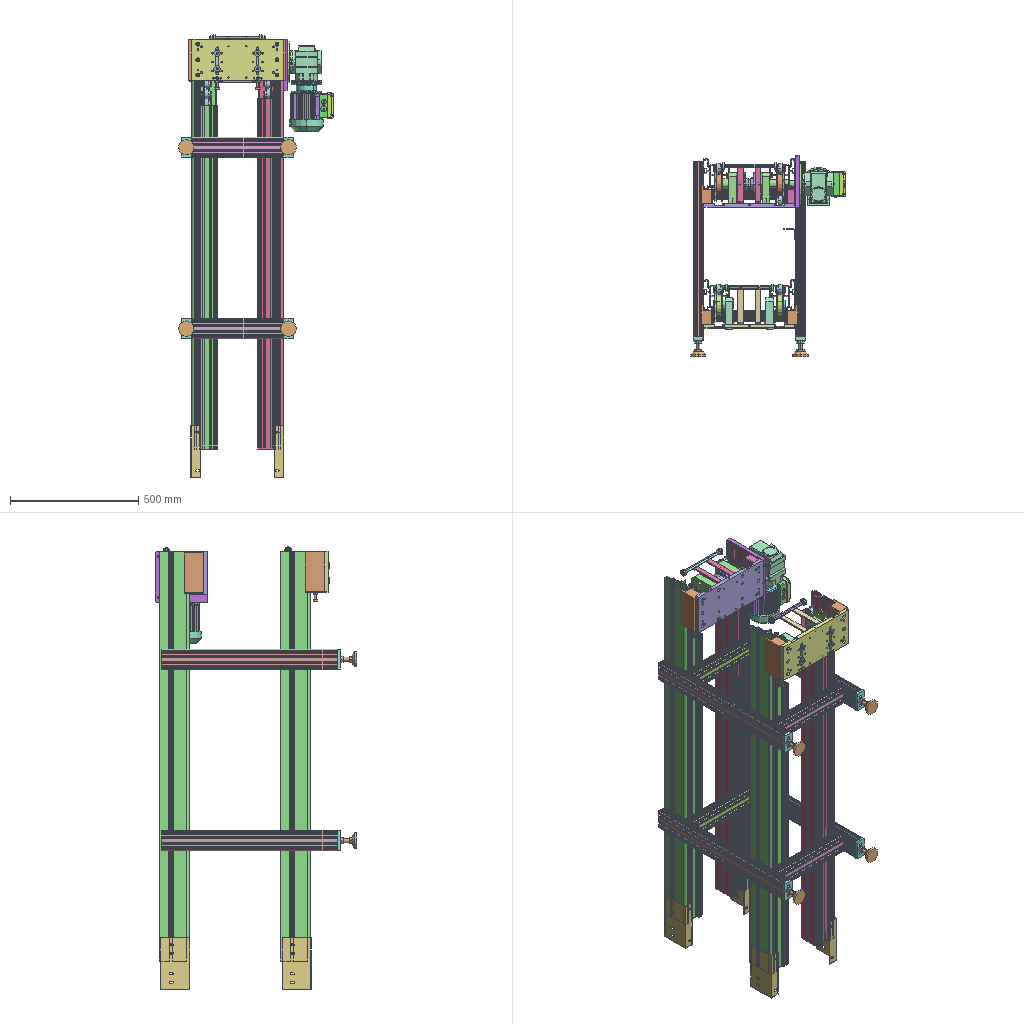Assembly | STEP file | 49 different items | 166 placed | box 603 x 786 x 1727 mm
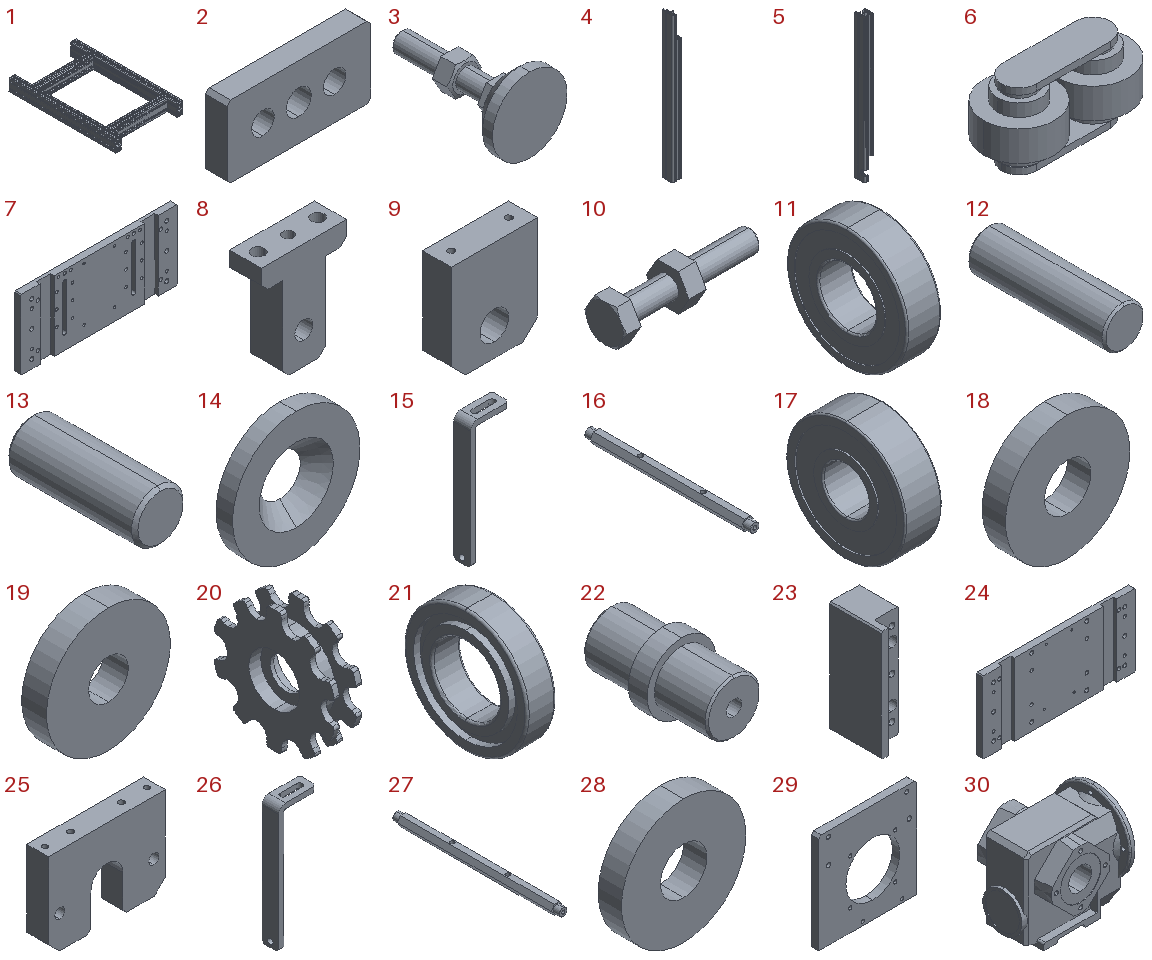Parts list (item | name | quantity | parent item | size | volume):
1 | PN_0014_default<as machined> | x2 | in PN_0013 | 439.002 x 686.5 x 80 mm | 2058365 mm3
2 | PN_0026_default | x4 | in PN_0013 | 80 x 12 x 40 mm | 33512 mm3
3 | PN_0021_default | x4 | in PN_0013 | 60 x 103 x 60 mm | 66755 mm3
4 | PN_0007_default | x2 | - | 100 x 118 x 1600 mm | 2634824 mm3
5 | PN_0009_default | x2 | - | 100 x 118 x 1600 mm | 2644329 mm3
6 | PN_0022_default | x64 | - | 74.7 x 36.6 x 38.9 mm | 50379 mm3
7 | PN_0031_default | x1 | in PN_0015 | 359 x 15 x 160 mm | 723262 mm3
8 | PN_0028_default | x2 | in PN_0015 | 40 x 15 x 50 mm | 16009 mm3
9 | PN_0020_default | x2 | in PN_0015 | 90 x 30 x 105 mm | 254060 mm3
10 | M10-60_RCB10-70 | x2 | in PN_0015 | 67 x 19.63 x 17 mm | 7820 mm3
11 | bearingB6004ZZ_default | x1 | in B6004ZZ_B6004ZZ | 12 x 42 x 42 mm | 12378 mm3
12 | PN_0030_default | x16 | in PN_0015 | 6 x 20 x 6 mm | 563.847 mm3
13 | PN_0023_default | x4 | in PN_0015 | 8 x 20 x 8 mm | 999.288 mm3
14 | PN_0018_default | x3 | in PN_0015 | 38.5 x 5 x 38.5 mm | 4599 mm3
15 | PN_0024_default | x2 | in PN_0015 | 45 x 20 x 148 mm | 20804 mm3
16 | PN_0002_default | x1 | in PN_0015 | 13.856 x 185 x 12 mm | 21503 mm3
17 | B6000ZZ_B6000ZZ | x4 | in PN_0015, PN_0029 | 8 x 26 x 26 mm | 3459 mm3
18 | PN_0004_default | x2 | in PN_0015 | 16 x 3 x 16 mm | 518.363 mm3
19 | PN_0001_default | x4 | in PN_0015 | 25 x 5 x 25 mm | 2203 mm3
20 | PN_0005_default | x2 | in PN_0015 | 30 x 129.474 x 133 mm | 166383 mm3
21 | B6006_B6006 | x4 | in PN_0015 | 13 x 55 x 55 mm | 18718 mm3
22 | PN_0010_default | x1 | in PN_0015 | 38 x 68.5 x 38 mm | 49766 mm3
23 | PN_0032_default | x3 | in PN_0015, PN_0029 | 44.75 x 75 x 160 mm | 399871 mm3
24 | PN_0016_default | x1 | in PN_0029 | 359 x 15 x 170 mm | 803822 mm3
25 | PN_0033_default | x2 | in PN_0029 | 161 x 30 x 120 mm | 471064 mm3
26 | PN_0006_default | x2 | in PN_0029 | 45 x 20 x 151 mm | 21164 mm3
27 | PN_0012_default | x1 | in PN_0029 | 13.856 x 210 x 12 mm | 24621 mm3
28 | PN_0008_default | x2 | in PN_0029 | 16 x 3 x 16 mm | 518.363 mm3
29 | PN_0011_default | x1 | in PN_0029 | 200 x 15 x 203 mm | 456778 mm3
30 | PRODUCT_NAME_32_default | x1 | in SAF37DR63L4-TF-n104-M1-B | 143 x 120 x 142 mm | 1389830 mm3
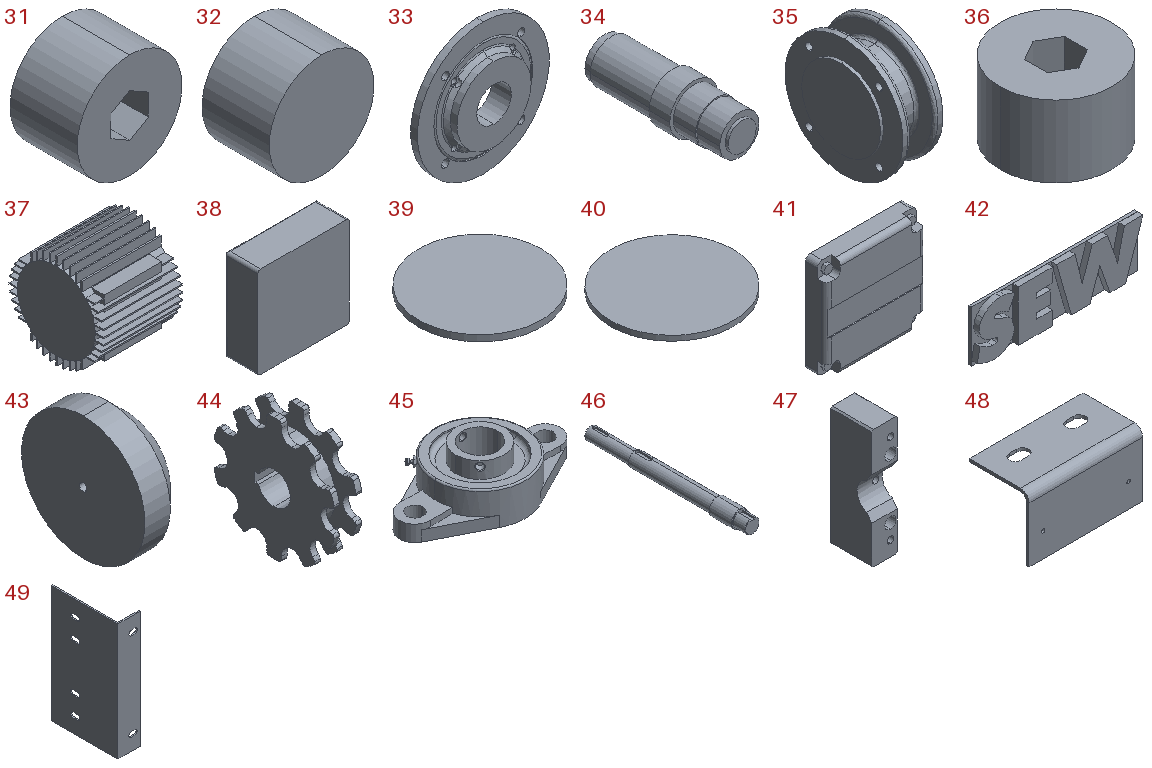31 | PRODUCT_NAME_33_default | x1 | in SAF37DR63L4-TF-n104-M1-B | 14 x 9 x 14 mm | 1299 mm3
32 | PRODUCT_NAME_34_default | x1 | in SAF37DR63L4-TF-n104-M1-B | 14 x 9 x 14 mm | 1299 mm3
33 | PRODUCT_NAME_35_default | x1 | in SAF37DR63L4-TF-n104-M1-B | 160 x 24 x 160 mm | 238568 mm3
34 | PRODUCT_NAME_36_default | x1 | in SAF37DR63L4-TF-n104-M1-B | 43 x 122.5 x 43 mm | 103084 mm3
35 | PRODUCT_NAME_37_default | x1 | in SAF37DR63L4-TF-n104-M1-B | 45 x 120 x 120 mm | 320577 mm3
36 | PRODUCT_NAME_38_default | x1 | in SAF37DR63L4-TF-n104-M1-B | 14 x 14 x 9 mm | 1299 mm3
37 | PRODUCT_NAME_39_default | x1 | in SAF37DR63L4-TF-n104-M1-B | 102 x 122 x 122 mm | 884304 mm3
38 | PRODUCT_NAME_40_default | x1 | in SAF37DR63L4-TF-n104-M1-B | 95 x 33 x 95 mm | 297490 mm3
39 | PRODUCT_NAME_41_default | x1 | in SAF37DR63L4-TF-n104-M1-B | 20 x 20 x 3.972 mm | 728.684 mm3
40 | PRODUCT_NAME_42_default | x1 | in SAF37DR63L4-TF-n104-M1-B | 24 x 24 x 4.478 mm | 1175 mm3
41 | PRODUCT_NAME_43_default | x1 | in SAF37DR63L4-TF-n104-M1-B | 100 x 21.5 x 100 mm | 204377 mm3
42 | PRODUCT_NAME_44_default | x1 | in SAF37DR63L4-TF-n104-M1-B | 58.086 x 3 x 18.091 mm | 2435 mm3
43 | PRODUCT_NAME_45_default | x1 | in SAF37DR63L4-TF-n104-M1-B | 47 x 132 x 132 mm | 566262 mm3
44 | PN_0003_default | x2 | in PN_0029 | 30 x 129.474 x 133 mm | 202077 mm3
45 | HDH35_HDH35 | x2 | in PN_0029 | 161 x 90 x 44.4 mm | 197699 mm3
46 | PN_0017_default | x1 | in PN_0029 | 42 x 401.5 x 42 mm | 377552 mm3
47 | PN_0025_default | x1 | in PN_0029 | 34 x 55 x 160 mm | 251328 mm3
48 | PN_0019_default | x1 | - | 80 x 42 x 45 mm | 12840 mm3
49 | PN_0027_default | x4 | - | 38 x 113 x 200 mm | 58277 mm3
Placements (level | parent | child | x y z in mm | rotation matrix by rows):
1 | subassembly 2 | PN_0013 | -225.021 25.346 -0.0 | 1 0 0 0 1 0 0 0 1
2 | PN_0013 | PN_0014_default<as machined> | -223.832 -352.823 20.0 | 1 0 0 0 1 0 0 0 1
2 | PN_0013 | PN_0026_default | -223.832 -364.823 0.0 | 0 0 1 0 1 0 -1 0 0
2 | PN_0013 | PN_0021_default | -223.832 -429.323 0.0 | 1 0 0 0 1 0 0 0 1
2 | PN_0013 | PN_0021_default | 175.168 -429.323 0.0 | -1 0 0 0 1 0 0 0 -1
2 | PN_0013 | PN_0026_default | 175.168 -364.823 0.0 | 0 0 1 0 1 0 -1 0 0
1 | subassembly 2 | PN_0007_default | -9538.032 1852.311 -470.0 | 1 0 0 0 1 0 0 0 1
1 | subassembly 2 | PN_0009_default | 9039.328 1852.311 1130.0 | -1 0 0 0 1 0 0 0 -1
1 | subassembly 2 | PN_0013 | -225.021 25.346 708.0 | 1 0 0 0 1 0 0 0 1
2 | PN_0013 | PN_0014_default<as machined> | -223.832 -352.823 20.0 | 1 0 0 0 1 0 0 0 1
2 | PN_0013 | PN_0026_default | -223.832 -364.823 0.0 | 0 0 1 0 1 0 -1 0 0
2 | PN_0013 | PN_0021_default | -223.832 -429.323 0.0 | 1 0 0 0 1 0 0 0 1
2 | PN_0013 | PN_0021_default | 175.168 -429.323 0.0 | -1 0 0 0 1 0 0 0 -1
2 | PN_0013 | PN_0026_default | 175.168 -364.823 0.0 | 0 0 1 0 1 0 -1 0 0
1 | subassembly 2 | PN_0022_default | -148.802 329.638 -410.0 | 0 0 1 0 1 0 -1 0 0
1 | subassembly 2 | PN_0022_default | -148.802 329.638 -332.0 | 0 0 1 0 1 0 -1 0 0
1 | subassembly 2 | PN_0022_default | -148.802 329.638 -254.0 | 0 0 1 0 1 0 -1 0 0
1 | subassembly 2 | PN_0022_default | -148.802 329.638 -176.0 | 0 0 1 0 1 0 -1 0 0
1 | subassembly 2 | PN_0022_default | -148.802 329.638 -98.0 | 0 0 1 0 1 0 -1 0 0
1 | subassembly 2 | PN_0022_default | -148.802 329.638 -20.0 | 0 0 1 0 1 0 -1 0 0
1 | subassembly 2 | PN_0022_default | -148.802 329.638 58.0 | 0 0 1 0 1 0 -1 0 0
1 | subassembly 2 | PN_0022_default | -148.802 329.638 136.0 | 0 0 1 0 1 0 -1 0 0
1 | subassembly 2 | PN_0022_default | -148.802 329.638 214.0 | 0 0 1 0 1 0 -1 0 0
1 | subassembly 2 | PN_0022_default | -148.802 329.638 292.0 | 0 0 1 0 1 0 -1 0 0
1 | subassembly 2 | PN_0022_default | -148.802 329.638 370.0 | 0 0 1 0 1 0 -1 0 0
1 | subassembly 2 | PN_0022_default | -148.802 329.638 448.0 | 0 0 1 0 1 0 -1 0 0
1 | subassembly 2 | PN_0022_default | -148.802 329.638 526.0 | 0 0 1 0 1 0 -1 0 0
1 | subassembly 2 | PN_0022_default | -148.802 329.638 604.0 | 0 0 1 0 1 0 -1 0 0
1 | subassembly 2 | PN_0022_default | -148.802 329.638 682.0 | 0 0 1 0 1 0 -1 0 0
1 | subassembly 2 | PN_0022_default | -148.802 329.638 760.0 | 0 0 1 0 1 0 -1 0 0
1 | subassembly 2 | PN_0022_default | -148.802 329.638 838.0 | 0 0 1 0 1 0 -1 0 0
1 | subassembly 2 | PN_0022_default | -148.802 329.638 916.0 | 0 0 1 0 1 0 -1 0 0
1 | subassembly 2 | PN_0022_default | -148.802 329.638 994.0 | 0 0 1 0 1 0 -1 0 0
1 | subassembly 2 | PN_0022_default | -148.802 329.638 1072.0 | 0 0 1 0 1 0 -1 0 0
1 | subassembly 2 | PN_0022_default | -388.802 329.638 -410.0 | 0 0 1 0 1 0 -1 0 0
1 | subassembly 2 | PN_0022_default | -388.802 329.638 -332.0 | 0 0 1 0 1 0 -1 0 0
1 | subassembly 2 | PN_0022_default | -388.802 329.638 -254.0 | 0 0 1 0 1 0 -1 0 0
1 | subassembly 2 | PN_0022_default | -388.802 329.638 1072.0 | 0 0 1 0 1 0 -1 0 0
1 | subassembly 2 | PN_0022_default | -388.802 329.638 -176.0 | 0 0 1 0 1 0 -1 0 0
1 | subassembly 2 | PN_0022_default | -388.802 329.638 -98.0 | 0 0 1 0 1 0 -1 0 0
1 | subassembly 2 | PN_0022_default | -388.802 329.638 -20.0 | 0 0 1 0 1 0 -1 0 0
1 | subassembly 2 | PN_0022_default | -388.802 329.638 58.0 | 0 0 1 0 1 0 -1 0 0
1 | subassembly 2 | PN_0022_default | -388.802 329.638 136.0 | 0 0 1 0 1 0 -1 0 0
1 | subassembly 2 | PN_0022_default | -388.802 329.638 214.0 | 0 0 1 0 1 0 -1 0 0
1 | subassembly 2 | PN_0022_default | -388.802 329.638 292.0 | 0 0 1 0 1 0 -1 0 0
1 | subassembly 2 | PN_0022_default | -388.802 329.638 370.0 | 0 0 1 0 1 0 -1 0 0
1 | subassembly 2 | PN_0022_default | -388.802 329.638 448.0 | 0 0 1 0 1 0 -1 0 0
1 | subassembly 2 | PN_0022_default | -388.802 329.638 526.0 | 0 0 1 0 1 0 -1 0 0
1 | subassembly 2 | PN_0022_default | -388.802 329.638 604.0 | 0 0 1 0 1 0 -1 0 0
1 | subassembly 2 | PN_0022_default | -388.802 329.638 682.0 | 0 0 1 0 1 0 -1 0 0
1 | subassembly 2 | PN_0022_default | -388.802 329.638 760.0 | 0 0 1 0 1 0 -1 0 0
1 | subassembly 2 | PN_0022_default | -388.802 329.638 838.0 | 0 0 1 0 1 0 -1 0 0
1 | subassembly 2 | PN_0022_default | -388.802 329.638 916.0 | 0 0 1 0 1 0 -1 0 0
1 | subassembly 2 | PN_0022_default | -388.802 329.638 994.0 | 0 0 1 0 1 0 -1 0 0
1 | subassembly 2 | PN_0022_default | -148.802 -142.362 916.0 | 0 0 1 0 1 0 -1 0 0
1 | subassembly 2 | PN_0022_default | -388.802 -142.362 916.0 | 0 0 1 0 1 0 -1 0 0
1 | subassembly 2 | PN_0022_default | -388.802 -142.362 994.0 | 0 0 1 0 1 0 -1 0 0
1 | subassembly 2 | PN_0022_default | -148.802 -142.362 994.0 | 0 0 1 0 1 0 -1 0 0
1 | subassembly 2 | PN_0022_default | -148.802 -142.362 1072.0 | 0 0 1 0 1 0 -1 0 0
1 | subassembly 2 | PN_0022_default | -388.802 -142.362 1072.0 | 0 0 1 0 1 0 -1 0 0
1 | subassembly 2 | PN_0022_default | -148.802 -142.362 -410.0 | 0 0 1 0 1 0 -1 0 0
1 | subassembly 2 | PN_0022_default | -148.802 -142.362 -332.0 | 0 0 1 0 1 0 -1 0 0
1 | subassembly 2 | PN_0022_default | -388.802 -142.362 -410.0 | 0 0 1 0 1 0 -1 0 0
1 | subassembly 2 | PN_0022_default | -388.802 -142.362 -332.0 | 0 0 1 0 1 0 -1 0 0
1 | subassembly 2 | PN_0022_default | -388.802 -142.362 -254.0 | 0 0 1 0 1 0 -1 0 0
1 | subassembly 2 | PN_0007_default | -9538.032 1380.311 -470.0 | 1 0 0 0 1 0 0 0 1
1 | subassembly 2 | PN_0009_default | 9039.328 1380.311 1130.0 | -1 0 0 0 1 0 0 0 -1
1 | subassembly 2 | PN_0022_default | -148.802 -142.362 214.0 | 0 0 1 0 1 0 -1 0 0
1 | subassembly 2 | PN_0022_default | -148.802 -142.362 292.0 | 0 0 1 0 1 0 -1 0 0
1 | subassembly 2 | PN_0022_default | -148.802 -142.362 370.0 | 0 0 1 0 1 0 -1 0 0
1 | subassembly 2 | PN_0022_default | -148.802 -142.362 448.0 | 0 0 1 0 1 0 -1 0 0
1 | subassembly 2 | PN_0022_default | -148.802 -142.362 526.0 | 0 0 1 0 1 0 -1 0 0
1 | subassembly 2 | PN_0022_default | -148.802 -142.362 604.0 | 0 0 1 0 1 0 -1 0 0
1 | subassembly 2 | PN_0022_default | -388.802 -142.362 214.0 | 0 0 1 0 1 0 -1 0 0
1 | subassembly 2 | PN_0022_default | -388.802 -142.362 292.0 | 0 0 1 0 1 0 -1 0 0
1 | subassembly 2 | PN_0022_default | -388.802 -142.362 370.0 | 0 0 1 0 1 0 -1 0 0
1 | subassembly 2 | PN_0022_default | -388.802 -142.362 448.0 | 0 0 1 0 1 0 -1 0 0
1 | subassembly 2 | PN_0022_default | -388.802 -142.362 526.0 | 0 0 1 0 1 0 -1 0 0
1 | subassembly 2 | PN_0022_default | -388.802 -142.362 604.0 | 0 0 1 0 1 0 -1 0 0
1 | subassembly 2 | PN_0015 | -251.774 -259.496 1050.0 | 1 0 0 0 -1 0 0 0 -1
2 | PN_0015 | PN_0031_default | 2.422 18.481 -0.0 | 1 0 0 0 1 0 0 0 1
2 | PN_0015 | PN_0028_default | -76.828 -6.519 80.0 | 1 0 0 0 0 1 0 -1 0
2 | PN_0015 | PN_0028_default | 81.672 -6.519 80.0 | 1 0 0 0 0 1 0 -1 0
2 | PN_0015 | PN_0020_default | -76.828 -34.019 5.0 | 0 1 0 0 0 1 1 0 -0
2 | PN_0015 | PN_0020_default | 81.672 -34.019 5.0 | 0 -1 0 0 0 1 -1 0 -0
2 | PN_0015 | M10-60_RCB10-70 | 81.672 -16.519 110.0 | 0 0.5 0.866 0 0.866 -0.5 -1 0 -0
2 | PN_0015 | M10-60_RCB10-70 | -76.828 -16.519 110.0 | 0 0.5 0.866 0 0.866 -0.5 -1 0 0
2 | PN_0015 | B6004ZZ_B6004ZZ | -76.828 -61.519 0.0 | 1 0 0 0 1 0 0 0 1
3 | B6004ZZ_B6004ZZ | bearingB6004ZZ_default | -0.0 -0.0 -0.0 | 1 0 0 0 1 0 0 0 1
2 | PN_0015 | PN_0030_default | -58.828 8.481 45.0 | 1 0 0 0 1 0 0 0 1
2 | PN_0015 | PN_0030_default | -58.828 8.481 10.0 | 1 0 0 0 1 0 0 0 1
2 | PN_0015 | PN_0030_default | -58.828 8.481 -25.0 | 1 0 0 0 1 0 0 0 1
2 | PN_0015 | PN_0030_default | -94.828 8.481 45.0 | 0.1404 0 0.9901 0 1 0 -0.9901 0 0.1404
2 | PN_0015 | PN_0030_default | -94.828 8.481 10.0 | 1 0 0 0 1 0 0 0 1
2 | PN_0015 | PN_0030_default | -94.828 8.481 -25.0 | 1 0 0 0 1 0 0 0 1
2 | PN_0015 | PN_0030_default | -62.828 8.481 72.5 | 1 0 0 0 1 0 0 0 1
2 | PN_0015 | PN_0030_default | -90.828 8.481 72.5 | 1 0 0 0 1 0 0 0 1
2 | PN_0015 | PN_0030_default | 95.672 8.481 72.5 | 0.9561 0 -0.2931 0 1 0 0.2931 0 0.9561
2 | PN_0015 | PN_0030_default | 67.672 8.481 72.5 | 0.9667 0 -0.2559 0 1 0 0.2559 0 0.9667
2 | PN_0015 | PN_0030_default | 99.672 8.481 45.0 | 0.4544 0 -0.8908 0 1 0 0.8908 0 0.4544
2 | PN_0015 | PN_0030_default | 99.672 8.481 10.0 | 1 0 0 0 1 0 0 0 1
2 | PN_0015 | PN_0030_default | 99.672 8.481 -25.0 | 1 0 0 0 1 0 0 0 1
2 | PN_0015 | PN_0030_default | 63.672 8.481 45.0 | 1 0 0 0 1 0 0 0 1
2 | PN_0015 | PN_0030_default | 63.672 8.481 10.0 | 1 0 0 0 1 0 0 0 1
2 | PN_0015 | PN_0030_default | 63.672 8.481 -25.0 | 1 0 0 0 1 0 0 0 1
2 | PN_0015 | PN_0023_default | 143.172 8.481 -50.0 | 1 0 0 0 1 0 0 0 1
2 | PN_0015 | PN_0023_default | 143.172 8.481 50.0 | 1 0 0 0 1 0 0 0 1
2 | PN_0015 | PN_0023_default | -138.328 8.481 50.0 | 0.2064 0 -0.9785 0 1 0 0.9785 0 0.2064
2 | PN_0015 | PN_0023_default | -138.328 8.481 -50.0 | 1 0 0 0 1 0 0 0 1
2 | PN_0015 | PN_0018_default | -59.828 -61.519 0.0 | 0 -1 0 -0.3818 0 -0.9242 0.9242 0 -0.3818
2 | PN_0015 | PN_0024_default | 27.422 -55.519 -55.5 | 0 1 0 0 0 1 1 0 -0
2 | PN_0015 | PN_0024_default | -42.578 -55.519 -55.5 | 0 1 0 0 0 1 1 0 -0
2 | PN_0015 | PN_0002_default | -90.078 -123.519 -84.0 | 0 1 0 -1 0 0 0 0 1
2 | PN_0015 | B6000ZZ_B6000ZZ | 94.922 -123.519 -84.0 | -1 0 0 0 -1 0 0 0 1
2 | PN_0015 | B6000ZZ_B6000ZZ | -82.078 -123.519 -84.0 | -1 0 0 0 -0.8372 0.5469 0 0.5469 0.8372
2 | PN_0015 | PN_0004_default | 94.922 -123.519 -84.0 | 0 1 0 -0.9644 0 -0.2646 -0.2646 0 0.9644
2 | PN_0015 | PN_0004_default | -90.078 -123.519 -84.0 | 0 -1 0 0.8671 0 0.4981 -0.4981 0 0.8671
2 | PN_0015 | PN_0001_default | 81.672 33.481 -25.0 | 1 0 0 0 1 0 0 0 1
2 | PN_0015 | PN_0001_default | 81.672 33.481 35.0 | 1 0 0 0 1 0 0 0 1
2 | PN_0015 | PN_0001_default | -76.828 33.481 -25.0 | 1 0 0 0 1 0 0 0 1
2 | PN_0015 | PN_0001_default | -76.828 33.481 35.0 | 1 0 0 0 1 0 0 0 1
2 | PN_0015 | PN_0005_default | 107.172 -56.519 5.0 | 1 0 0 0 0.9423 0.3348 0 -0.3348 0.9423
2 | PN_0015 | B6006_B6006 | 124.172 -56.519 5.0 | 1 0 0 0 0.9955 -0.09481 0 0.09481 0.9955
2 | PN_0015 | B6006_B6006 | 107.172 -56.519 5.0 | 1 0 0 0 0.9955 -0.09481 0 0.09481 0.9955
2 | PN_0015 | PN_0018_default | 142.172 -56.519 5.0 | 0 -1 0 0.5523 0 0.8337 -0.8337 0 0.5523
2 | PN_0015 | PN_0018_default | -137.328 -56.519 5.0 | 0 1 0 0.5523 0 -0.8337 -0.8337 0 -0.5523
2 | PN_0015 | PN_0005_default | -102.328 -56.519 5.0 | -1 0 0 0 0.9423 -0.3348 0 -0.3348 -0.9423
2 | PN_0015 | PN_0010_default | -102.328 -56.519 5.0 | 0 1 0 0.9968 0 0.08002 0.08002 0 -0.9968
2 | PN_0015 | B6006_B6006 | -102.328 -56.519 5.0 | -1 0 0 0 0.9955 0.09481 0 0.09481 -0.9955
2 | PN_0015 | B6006_B6006 | -119.328 -56.519 5.0 | -1 0 0 0 0.9955 0.09481 0 0.09481 -0.9955
2 | PN_0015 | PN_0032_default | -164.703 -56.519 -0.0 | 1 0 0 0 1 0 0 0 1
2 | PN_0015 | PN_0032_default | 169.547 -56.519 -0.0 | -1 0 0 0 1 0 0 0 -1
1 | subassembly 2 | PN_0029 | -265.491 217.569 1045.0 | 1 0 0 0 -1 0 0 0 -1
2 | PN_0029 | PN_0016_default | 16.139 23.546 -0.0 | 1 0 0 0 1 0 0 0 1
2 | PN_0029 | PN_0033_default | -63.861 -36.454 4.5 | 0 1 0 0 0 1 1 0 -0
2 | PN_0029 | PN_0033_default | 96.139 -36.454 4.5 | 0 -1 0 0 0 1 -1 0 0
2 | PN_0029 | PN_0006_default | -28.861 -51.954 -57.5 | 0 1 0 0 0 1 1 0 -0
2 | PN_0029 | PN_0006_default | 41.139 -51.954 -57.5 | 0 1 0 0 0 1 1 0 -0
2 | PN_0029 | PN_0012_default | -88.861 -121.454 -86.0 | 0 1 0 -1 0 0 0 0 1
2 | PN_0029 | B6000ZZ_B6000ZZ | -88.861 -121.454 -86.0 | 1 0 0 0 0 -1 0 1 -0
2 | PN_0029 | B6000ZZ_B6000ZZ | 113.139 -121.454 -86.0 | 1 0 0 0 0.9207 0.3904 0 -0.3904 0.9207
2 | PN_0029 | PN_0008_default | -88.861 -121.454 -86.0 | 0 -1 0 0.922 0 -0.3872 0.3872 0 0.922
2 | PN_0029 | PN_0008_default | 121.139 -121.454 -86.0 | 0 1 0 -0.879 0 0.4768 0.4768 0 0.879
2 | PN_0029 | PN_0011_default | 195.639 -67.954 15.0 | 0 1 0 0 0 -1 -1 0 -0
2 | PN_0029 | SAF37DR63L4-TF-n104-M1-B | 342.639 -51.454 4.5 | 0 -1 0 0 0 -1 1 0 -0
3 | SAF37DR63L4-TF-n104-M1-B | PRODUCT_NAME_32_default | -0.0 -0.0 -0.0 | 1 0 0 0 1 0 0 0 1
3 | SAF37DR63L4-TF-n104-M1-B | PRODUCT_NAME_33_default | -0.0 -0.0 -0.0 | 1 0 0 0 1 0 0 0 1
3 | SAF37DR63L4-TF-n104-M1-B | PRODUCT_NAME_34_default | -0.0 -0.0 -0.0 | 1 0 0 0 1 0 0 0 1
3 | SAF37DR63L4-TF-n104-M1-B | PRODUCT_NAME_35_default | -0.0 -0.0 -0.0 | 1 0 0 0 1 0 0 0 1
3 | SAF37DR63L4-TF-n104-M1-B | PRODUCT_NAME_36_default | -0.0 -0.0 -0.0 | 1 0 0 0 1 0 0 0 1
3 | SAF37DR63L4-TF-n104-M1-B | PRODUCT_NAME_37_default | 0.0 16.695 40.305 | 1 0 0 0 0.7071 0.7071 0 -0.7071 0.7071
3 | SAF37DR63L4-TF-n104-M1-B | PRODUCT_NAME_38_default | -0.0 -0.0 -0.0 | 1 0 0 0 1 0 0 0 1
3 | SAF37DR63L4-TF-n104-M1-B | PRODUCT_NAME_39_default | -0.0 -0.0 -0.0 | 1 0 0 0 1 0 0 0 1
3 | SAF37DR63L4-TF-n104-M1-B | PRODUCT_NAME_40_default | -0.0 -0.0 -0.0 | 1 0 0 0 1 0 0 0 1
3 | SAF37DR63L4-TF-n104-M1-B | PRODUCT_NAME_41_default | -0.0 -0.0 -0.0 | 1 0 0 0 1 0 0 0 1
3 | SAF37DR63L4-TF-n104-M1-B | PRODUCT_NAME_42_default | -0.0 -0.0 -0.0 | 1 0 0 0 1 0 0 0 1
3 | SAF37DR63L4-TF-n104-M1-B | PRODUCT_NAME_43_default | -0.0 -0.0 -0.0 | 1 0 0 0 1 0 0 0 1
3 | SAF37DR63L4-TF-n104-M1-B | PRODUCT_NAME_44_default | -0.0 -0.0 -0.0 | 1 0 0 0 1 0 0 0 1
3 | SAF37DR63L4-TF-n104-M1-B | PRODUCT_NAME_45_default | -0.0 -0.0 -0.0 | 1 0 0 0 1 0 0 0 1
2 | PN_0029 | PN_0003_default | -118.861 -51.454 4.5 | 1 0 0 0 0.5222 0.8529 0 -0.8529 0.5222
2 | PN_0029 | PN_0003_default | 151.139 -51.454 4.5 | -1 0 0 0 0.5222 -0.8529 0 -0.8529 -0.5222
2 | PN_0029 | HDH35_HDH35 | -11.661 -51.454 4.5 | 0 0 1 0 1 0 -1 0 -0
2 | PN_0029 | HDH35_HDH35 | 43.939 -51.415 4.5 | 0 0 -1 0 -1 0 -1 0 -0
2 | PN_0029 | PN_0017_default | -118.861 -51.454 4.5 | 0 1 0 0.8529 0 0.5222 0.5222 0 -0.8529
2 | PN_0029 | PN_0032_default | -150.986 -51.454 -0.0 | 1 0 0 0 1 0 0 0 1
2 | PN_0029 | PN_0025_default | 178.639 -31.454 -0.0 | -1 0 0 0 1 0 0 0 -1
1 | subassembly 2 | PN_0019_default | -71.852 93.534 -40.0 | 0 0 1 0 -1 0 1 0 -0
1 | subassembly 2 | PN_0027_default | -430.852 303.523 -480.0 | 1 0 0 0 1 0 0 0 1
1 | subassembly 2 | PN_0027_default | -67.852 303.523 -480.0 | -1 0 0 0 1 0 0 0 -1
1 | subassembly 2 | PN_0027_default | -430.852 -169.477 -480.0 | 1 0 0 0 1 0 0 0 1
1 | subassembly 2 | PN_0027_default | -67.852 -169.477 -480.0 | -1 0 0 0 1 0 0 0 -1
1 | subassembly 2 | PN_0022_default | -148.802 204.638 1072.0 | 0 0 1 0 1 0 -1 0 0